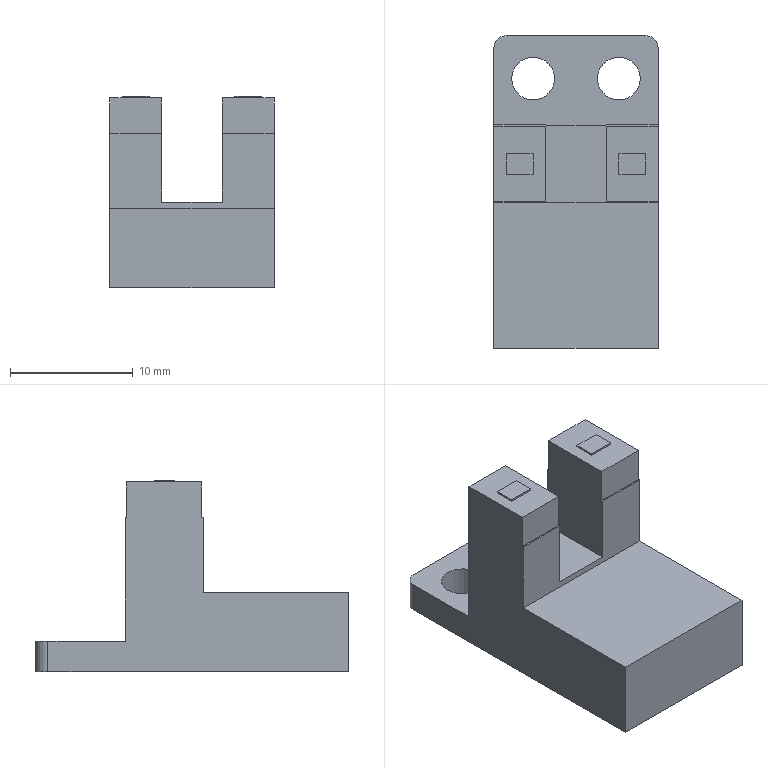Part | SolidWorks | features BaseBody 1 | 1 solid | 38 faces | box 13.4 x 25.5 x 15.65 mm | volume 2274 mm3 | plane 32 | cylinder 6 | commonest cylinder face diameters 3.5 x4 2 x2
STEP:
#1=CARTESIAN_POINT('',(304.797,1020.806,-399.345));
#2=VERTEX_POINT('',#1);
#3=CARTESIAN_POINT('',(301.297,1020.806,-399.345));
#4=VERTEX_POINT('',#3);
#5=CARTESIAN_POINT('',(303.047,1020.806,-399.345));
#6=DIRECTION('',(0.,0.,-1.));
#7=DIRECTION('',(-1.,0.,0.));
#8=AXIS2_PLACEMENT_3D('',#5,#6,#7);
#9=CIRCLE('',#8,1.75);
#10=EDGE_CURVE('',#2,#4,#9,.T.);
#11=ORIENTED_EDGE('',*,*,#10,.F.);
#12=CARTESIAN_POINT('',(304.797,1020.806,-401.845));
#13=VERTEX_POINT('',#12);
#14=CARTESIAN_POINT('',(304.797,1020.806,-344.345));
#15=DIRECTION('',(0.,0.,-1.));
#16=VECTOR('',#15,1000.);
#17=LINE('',#14,#16);
#18=EDGE_CURVE('',#2,#13,#17,.T.);
#19=ORIENTED_EDGE('',*,*,#18,.T.);
#20=CARTESIAN_POINT('',(301.297,1020.806,-401.845));
#21=VERTEX_POINT('',#20);
#22=CARTESIAN_POINT('',(303.047,1020.806,-401.845));
#23=DIRECTION('',(0.,0.,1.));
#24=DIRECTION('',(-1.,0.,0.));
#25=AXIS2_PLACEMENT_3D('',#22,#23,#24);
#26=CIRCLE('',#25,1.75);
#27=EDGE_CURVE('',#21,#13,#26,.T.);
#28=ORIENTED_EDGE('',*,*,#27,.F.);
#29=CARTESIAN_POINT('',(301.297,1020.806,-344.345));
#30=DIRECTION('',(0.,0.,-1.));
#31=VECTOR('',#30,1000.);
#32=LINE('',#29,#31);
#33=EDGE_CURVE('',#4,#21,#32,.T.);
#34=ORIENTED_EDGE('',*,*,#33,.F.);
#35=EDGE_LOOP('',(#11,#19,#28,#34));
#36=FACE_OUTER_BOUND('',#35,.T.);
#37=CARTESIAN_POINT('',(303.047,1020.806,-344.345));
#38=DIRECTION('',(0.,0.,-1.));
#39=DIRECTION('',(-1.,0.,0.));
#40=AXIS2_PLACEMENT_3D('',#37,#38,#39);
#41=CYLINDRICAL_SURFACE('',#40,1.75);
#42=ADVANCED_FACE('',(#36),#41,.F.);
#43=CARTESIAN_POINT('',(297.797,1020.806,-399.345));
#44=VERTEX_POINT('',#43);
#45=CARTESIAN_POINT('',(294.297,1020.806,-399.345));
#46=VERTEX_POINT('',#45);
#47=CARTESIAN_POINT('',(296.047,1020.806,-399.345));
#48=DIRECTION('',(0.,0.,-1.));
#49=DIRECTION('',(-1.,0.,0.));
#50=AXIS2_PLACEMENT_3D('',#47,#48,#49);
#51=CIRCLE('',#50,1.75);
#52=EDGE_CURVE('',#44,#46,#51,.T.);
#53=ORIENTED_EDGE('',*,*,#52,.F.);
#54=CARTESIAN_POINT('',(297.797,1020.806,-401.845));
#55=VERTEX_POINT('',#54);
#56=CARTESIAN_POINT('',(297.797,1020.806,-344.345));
#57=DIRECTION('',(0.,0.,-1.));
#58=VECTOR('',#57,1000.);
#59=LINE('',#56,#58);
#60=EDGE_CURVE('',#44,#55,#59,.T.);
#61=ORIENTED_EDGE('',*,*,#60,.T.);
#62=CARTESIAN_POINT('',(294.297,1020.806,-401.845));
#63=VERTEX_POINT('',#62);
#64=CARTESIAN_POINT('',(296.047,1020.806,-401.845));
#65=DIRECTION('',(0.,0.,1.));
#66=DIRECTION('',(-1.,0.,0.));
#67=AXIS2_PLACEMENT_3D('',#64,#65,#66);
#68=CIRCLE('',#67,1.75);
#69=EDGE_CURVE('',#63,#55,#68,.T.);
#70=ORIENTED_EDGE('',*,*,#69,.F.);
#71=CARTESIAN_POINT('',(294.297,1020.806,-344.345));
#72=DIRECTION('',(0.,0.,-1.));
#73=VECTOR('',#72,1000.);
#74=LINE('',#71,#73);
#75=EDGE_CURVE('',#46,#63,#74,.T.);
#76=ORIENTED_EDGE('',*,*,#75,.F.);
#77=EDGE_LOOP('',(#53,#61,#70,#76));
#78=FACE_OUTER_BOUND('',#77,.T.);
#79=CARTESIAN_POINT('',(296.047,1020.806,-344.345));
#80=DIRECTION('',(0.,0.,-1.));
#81=DIRECTION('',(-1.,0.,0.));
#82=AXIS2_PLACEMENT_3D('',#79,#80,#81);
#83=CYLINDRICAL_SURFACE('',#82,1.75);
#84=ADVANCED_FACE('',(#78),#83,.F.);
#85=ORIENTED_EDGE('',*,*,#27,.T.);
#86=CARTESIAN_POINT('',(303.047,1020.806,-401.845));
#87=DIRECTION('',(0.,0.,1.));
#88=DIRECTION('',(-1.,0.,0.));
#89=AXIS2_PLACEMENT_3D('',#86,#87,#88);
#90=CIRCLE('',#89,1.75);
#91=EDGE_CURVE('',#13,#21,#90,.T.);
#92=ORIENTED_EDGE('',*,*,#91,.T.);
#93=EDGE_LOOP('',(#85,#92));
#94=FACE_BOUND('',#93,.T.);
#95=ORIENTED_EDGE('',*,*,#69,.T.);
#96=CARTESIAN_POINT('',(296.047,1020.806,-401.845));
#97=DIRECTION('',(0.,0.,1.));
#98=DIRECTION('',(-1.,0.,0.));
#99=AXIS2_PLACEMENT_3D('',#96,#97,#98);
#100=CIRCLE('',#99,1.75);
#101=EDGE_CURVE('',#55,#63,#100,.T.);
#102=ORIENTED_EDGE('',*,*,#101,.T.);
#103=EDGE_LOOP('',(#95,#102));
#104=FACE_BOUND('',#103,.T.);
#105=CARTESIAN_POINT('',(292.847,1023.306,-401.845));
#106=VERTEX_POINT('',#105);
#107=CARTESIAN_POINT('',(293.847,1024.306,-401.845));
#108=VERTEX_POINT('',#107);
#109=CARTESIAN_POINT('',(293.847,1023.306,-401.845));
#110=DIRECTION('',(0.,0.,-1.));
#111=DIRECTION('',(1.,0.,0.));
#112=AXIS2_PLACEMENT_3D('',#109,#110,#111);
#113=CIRCLE('',#112,1.);
#114=EDGE_CURVE('',#106,#108,#113,.T.);
#115=ORIENTED_EDGE('',*,*,#114,.T.);
#116=CARTESIAN_POINT('',(305.247,1024.306,-401.845));
#117=VERTEX_POINT('',#116);
#118=CARTESIAN_POINT('',(306.247,1024.306,-401.845));
#119=DIRECTION('',(1.,0.,0.));
#120=VECTOR('',#119,1000.);
#121=LINE('',#118,#120);
#122=EDGE_CURVE('',#108,#117,#121,.T.);
#123=ORIENTED_EDGE('',*,*,#122,.T.);
#124=CARTESIAN_POINT('',(306.247,1023.306,-401.845));
#125=VERTEX_POINT('',#124);
#126=CARTESIAN_POINT('',(305.247,1023.306,-401.845));
#127=DIRECTION('',(0.,0.,-1.));
#128=DIRECTION('',(-1.,0.,0.));
#129=AXIS2_PLACEMENT_3D('',#126,#127,#128);
#130=CIRCLE('',#129,1.);
#131=EDGE_CURVE('',#117,#125,#130,.T.);
#132=ORIENTED_EDGE('',*,*,#131,.T.);
#133=CARTESIAN_POINT('',(306.247,998.806,-401.845));
#134=VERTEX_POINT('',#133);
#135=CARTESIAN_POINT('',(306.247,998.806,-401.845));
#136=DIRECTION('',(0.,-1.,0.));
#137=VECTOR('',#136,1000.);
#138=LINE('',#135,#137);
#139=EDGE_CURVE('',#125,#134,#138,.T.);
#140=ORIENTED_EDGE('',*,*,#139,.T.);
#141=CARTESIAN_POINT('',(292.847,998.806,-401.845));
#142=VERTEX_POINT('',#141);
#143=CARTESIAN_POINT('',(306.247,998.806,-401.845));
#144=DIRECTION('',(-1.,0.,0.));
#145=VECTOR('',#144,1000.);
#146=LINE('',#143,#145);
#147=EDGE_CURVE('',#134,#142,#146,.T.);
#148=ORIENTED_EDGE('',*,*,#147,.T.);
#149=CARTESIAN_POINT('',(292.847,998.806,-401.845));
#150=DIRECTION('',(0.,1.,0.));
#151=VECTOR('',#150,1000.);
#152=LINE('',#149,#151);
#153=EDGE_CURVE('',#142,#106,#152,.T.);
#154=ORIENTED_EDGE('',*,*,#153,.T.);
#155=EDGE_LOOP('',(#115,#123,#132,#140,#148,#154));
#156=FACE_OUTER_BOUND('',#155,.T.);
#157=CARTESIAN_POINT('',(306.247,998.806,-401.845));
#158=DIRECTION('',(0.,0.,-1.));
#159=DIRECTION('',(-1.,0.,0.));
#160=AXIS2_PLACEMENT_3D('',#157,#158,#159);
#161=PLANE('',#160);
#162=ADVANCED_FACE('',(#94,#104,#156),#161,.T.);
#163=ORIENTED_EDGE('',*,*,#18,.F.);
#164=CARTESIAN_POINT('',(303.047,1020.806,-399.345));
#165=DIRECTION('',(0.,0.,-1.));
#166=DIRECTION('',(-1.,0.,0.));
#167=AXIS2_PLACEMENT_3D('',#164,#165,#166);
#168=CIRCLE('',#167,1.75);
#169=EDGE_CURVE('',#4,#2,#168,.T.);
#170=ORIENTED_EDGE('',*,*,#169,.F.);
#171=ORIENTED_EDGE('',*,*,#33,.T.);
#172=ORIENTED_EDGE('',*,*,#91,.F.);
#173=EDGE_LOOP('',(#163,#170,#171,#172));
#174=FACE_OUTER_BOUND('',#173,.T.);
#175=CARTESIAN_POINT('',(303.047,1020.806,-344.345));
#176=DIRECTION('',(0.,0.,-1.));
#177=DIRECTION('',(-1.,0.,0.));
#178=AXIS2_PLACEMENT_3D('',#175,#176,#177);
#179=CYLINDRICAL_SURFACE('',#178,1.75);
#180=ADVANCED_FACE('',(#174),#179,.F.);
#181=ORIENTED_EDGE('',*,*,#60,.F.);
#182=CARTESIAN_POINT('',(296.047,1020.806,-399.345));
#183=DIRECTION('',(0.,0.,-1.));
#184=DIRECTION('',(-1.,0.,0.));
#185=AXIS2_PLACEMENT_3D('',#182,#183,#184);
#186=CIRCLE('',#185,1.75);
#187=EDGE_CURVE('',#46,#44,#186,.T.);
#188=ORIENTED_EDGE('',*,*,#187,.F.);
#189=ORIENTED_EDGE('',*,*,#75,.T.);
#190=ORIENTED_EDGE('',*,*,#101,.F.);
#191=EDGE_LOOP('',(#181,#188,#189,#190));
#192=FACE_OUTER_BOUND('',#191,.T.);
#193=CARTESIAN_POINT('',(296.047,1020.806,-344.345));
#194=DIRECTION('',(0.,0.,-1.));
#195=DIRECTION('',(-1.,0.,0.));
#196=AXIS2_PLACEMENT_3D('',#193,#194,#195);
#197=CYLINDRICAL_SURFACE('',#196,1.75);
#198=ADVANCED_FACE('',(#192),#197,.F.);
#199=CARTESIAN_POINT('',(293.847,1024.306,-399.345));
#200=VERTEX_POINT('',#199);
#201=CARTESIAN_POINT('',(293.847,1024.306,-444.345));
#202=DIRECTION('',(0.,0.,1.));
#203=VECTOR('',#202,1000.);
#204=LINE('',#201,#203);
#205=EDGE_CURVE('',#108,#200,#204,.T.);
#206=ORIENTED_EDGE('',*,*,#205,.T.);
#207=CARTESIAN_POINT('',(305.247,1024.306,-399.345));
#208=VERTEX_POINT('',#207);
#209=CARTESIAN_POINT('',(357.247,1024.306,-399.345));
#210=DIRECTION('',(1.,0.,0.));
#211=VECTOR('',#210,1000.);
#212=LINE('',#209,#211);
#213=EDGE_CURVE('',#200,#208,#212,.T.);
#214=ORIENTED_EDGE('',*,*,#213,.T.);
#215=CARTESIAN_POINT('',(305.247,1024.306,-444.345));
#216=DIRECTION('',(0.,0.,-1.));
#217=VECTOR('',#216,1000.);
#218=LINE('',#215,#217);
#219=EDGE_CURVE('',#208,#117,#218,.T.);
#220=ORIENTED_EDGE('',*,*,#219,.T.);
#221=ORIENTED_EDGE('',*,*,#122,.F.);
#222=EDGE_LOOP('',(#206,#214,#220,#221));
#223=FACE_OUTER_BOUND('',#222,.T.);
#224=CARTESIAN_POINT('',(357.247,1024.306,-444.345));
#225=DIRECTION('',(0.,1.,0.));
#226=DIRECTION('',(0.,0.,1.));
#227=AXIS2_PLACEMENT_3D('',#224,#225,#226);
#228=PLANE('',#227);
#229=ADVANCED_FACE('',(#223),#228,.T.);
#230=ORIENTED_EDGE('',*,*,#205,.F.);
#231=ORIENTED_EDGE('',*,*,#114,.F.);
#232=CARTESIAN_POINT('',(292.847,1023.306,-399.345));
#233=VERTEX_POINT('',#232);
#234=CARTESIAN_POINT('',(292.847,1023.306,-444.345));
#235=DIRECTION('',(0.,0.,1.));
#236=VECTOR('',#235,1000.);
#237=LINE('',#234,#236);
#238=EDGE_CURVE('',#106,#233,#237,.T.);
#239=ORIENTED_EDGE('',*,*,#238,.T.);
#240=CARTESIAN_POINT('',(293.847,1023.306,-399.345));
#241=DIRECTION('',(0.,0.,-1.));
#242=DIRECTION('',(1.,0.,0.));
#243=AXIS2_PLACEMENT_3D('',#240,#241,#242);
#244=CIRCLE('',#243,1.);
#245=EDGE_CURVE('',#233,#200,#244,.T.);
#246=ORIENTED_EDGE('',*,*,#245,.T.);
#247=EDGE_LOOP('',(#230,#231,#239,#246));
#248=FACE_OUTER_BOUND('',#247,.T.);
#249=CARTESIAN_POINT('',(293.847,1023.306,-444.345));
#250=DIRECTION('',(0.,0.,1.));
#251=DIRECTION('',(1.,0.,0.));
#252=AXIS2_PLACEMENT_3D('',#249,#250,#251);
#253=CYLINDRICAL_SURFACE('',#252,1.);
#254=ADVANCED_FACE('',(#248),#253,.T.);
#255=CARTESIAN_POINT('',(292.847,1017.006,-389.245));
#256=VERTEX_POINT('',#255);
#257=CARTESIAN_POINT('',(292.847,1017.006,-399.345));
#258=VERTEX_POINT('',#257);
#259=CARTESIAN_POINT('',(292.847,1017.006,-401.845));
#260=DIRECTION('',(0.,0.,-1.));
#261=VECTOR('',#260,1000.);
#262=LINE('',#259,#261);
#263=EDGE_CURVE('',#256,#258,#262,.T.);
#264=ORIENTED_EDGE('',*,*,#263,.T.);
#265=CARTESIAN_POINT('',(292.847,998.806,-399.345));
#266=DIRECTION('',(0.,1.,0.));
#267=VECTOR('',#266,1000.);
#268=LINE('',#265,#267);
#269=EDGE_CURVE('',#258,#233,#268,.T.);
#270=ORIENTED_EDGE('',*,*,#269,.T.);
#271=ORIENTED_EDGE('',*,*,#238,.F.);
#272=ORIENTED_EDGE('',*,*,#153,.F.);
#273=CARTESIAN_POINT('',(292.847,998.806,-395.345));
#274=VERTEX_POINT('',#273);
#275=CARTESIAN_POINT('',(292.847,998.806,-401.845));
#276=DIRECTION('',(0.,0.,1.));
#277=VECTOR('',#276,1000.);
#278=LINE('',#275,#277);
#279=EDGE_CURVE('',#142,#274,#278,.T.);
#280=ORIENTED_EDGE('',*,*,#279,.T.);
#281=CARTESIAN_POINT('',(292.847,1010.656,-395.345));
#282=VERTEX_POINT('',#281);
#283=CARTESIAN_POINT('',(292.847,998.806,-395.345));
#284=DIRECTION('',(0.,1.,0.));
#285=VECTOR('',#284,1000.);
#286=LINE('',#283,#285);
#287=EDGE_CURVE('',#274,#282,#286,.T.);
#288=ORIENTED_EDGE('',*,*,#287,.T.);
#289=CARTESIAN_POINT('',(292.847,1010.656,-389.245));
#290=VERTEX_POINT('',#289);
#291=CARTESIAN_POINT('',(292.847,1010.656,-401.845));
#292=DIRECTION('',(0.,0.,1.));
#293=VECTOR('',#292,1000.);
#294=LINE('',#291,#293);
#295=EDGE_CURVE('',#282,#290,#294,.T.);
#296=ORIENTED_EDGE('',*,*,#295,.T.);
#297=CARTESIAN_POINT('',(292.847,1010.756,-389.245));
#298=VERTEX_POINT('',#297);
#299=CARTESIAN_POINT('',(292.847,998.806,-389.245));
#300=DIRECTION('',(0.,1.,0.));
#301=VECTOR('',#300,1000.);
#302=LINE('',#299,#301);
#303=EDGE_CURVE('',#290,#298,#302,.T.);
#304=ORIENTED_EDGE('',*,*,#303,.T.);
#305=CARTESIAN_POINT('',(292.847,1010.756,-386.345));
#306=VERTEX_POINT('',#305);
#307=CARTESIAN_POINT('',(292.847,1010.756,-401.845));
#308=DIRECTION('',(0.,0.,1.));
#309=VECTOR('',#308,1000.);
#310=LINE('',#307,#309);
#311=EDGE_CURVE('',#298,#306,#310,.T.);
#312=ORIENTED_EDGE('',*,*,#311,.T.);
#313=CARTESIAN_POINT('',(292.847,1016.906,-386.345));
#314=VERTEX_POINT('',#313);
#315=CARTESIAN_POINT('',(292.847,998.806,-386.345));
#316=DIRECTION('',(0.,1.,0.));
#317=VECTOR('',#316,1000.);
#318=LINE('',#315,#317);
#319=EDGE_CURVE('',#306,#314,#318,.T.);
#320=ORIENTED_EDGE('',*,*,#319,.T.);
#321=CARTESIAN_POINT('',(292.847,1016.906,-389.245));
#322=VERTEX_POINT('',#321);
#323=CARTESIAN_POINT('',(292.847,1016.906,-401.845));
#324=DIRECTION('',(0.,0.,-1.));
#325=VECTOR('',#324,1000.);
#326=LINE('',#323,#325);
#327=EDGE_CURVE('',#314,#322,#326,.T.);
#328=ORIENTED_EDGE('',*,*,#327,.T.);
#329=CARTESIAN_POINT('',(292.847,998.806,-389.245));
#330=DIRECTION('',(0.,1.,0.));
#331=VECTOR('',#330,1000.);
#332=LINE('',#329,#331);
#333=EDGE_CURVE('',#322,#256,#332,.T.);
#334=ORIENTED_EDGE('',*,*,#333,.T.);
#335=EDGE_LOOP('',(#264,#270,#271,#272,#280,#288,#296,#304,#312,#320,#328,#334));
#336=FACE_OUTER_BOUND('',#335,.T.);
#337=CARTESIAN_POINT('',(292.847,998.806,-401.845));
#338=DIRECTION('',(-1.,0.,0.));
#339=DIRECTION('',(0.,0.,1.));
#340=AXIS2_PLACEMENT_3D('',#337,#338,#339);
#341=PLANE('',#340);
#342=ADVANCED_FACE('',(#336),#341,.T.);
#343=ORIENTED_EDGE('',*,*,#279,.F.);
#344=ORIENTED_EDGE('',*,*,#147,.F.);
#345=CARTESIAN_POINT('',(306.247,998.806,-395.345));
#346=VERTEX_POINT('',#345);
#347=CARTESIAN_POINT('',(306.247,998.806,-444.345));
#348=DIRECTION('',(0.,0.,-1.));
#349=VECTOR('',#348,1000.);
#350=LINE('',#347,#349);
#351=EDGE_CURVE('',#346,#134,#350,.T.);
#352=ORIENTED_EDGE('',*,*,#351,.F.);
#353=CARTESIAN_POINT('',(357.247,998.806,-395.345));
#354=DIRECTION('',(1.,0.,0.));
#355=VECTOR('',#354,1000.);
#356=LINE('',#353,#355);
#357=EDGE_CURVE('',#274,#346,#356,.T.);
#358=ORIENTED_EDGE('',*,*,#357,.F.);
#359=EDGE_LOOP('',(#343,#344,#352,#358));
#360=FACE_OUTER_BOUND('',#359,.T.);
#361=CARTESIAN_POINT('',(357.247,998.806,-444.345));
#362=DIRECTION('',(0.,1.,0.));
#363=DIRECTION('',(0.,0.,1.));
#364=AXIS2_PLACEMENT_3D('',#361,#362,#363);
#365=PLANE('',#364);
#366=ADVANCED_FACE('',(#360),#365,.F.);
#367=ORIENTED_EDGE('',*,*,#351,.T.);
#368=ORIENTED_EDGE('',*,*,#139,.F.);
#369=CARTESIAN_POINT('',(306.247,1023.306,-399.345));
#370=VERTEX_POINT('',#369);
#371=CARTESIAN_POINT('',(306.247,1023.306,-386.345));
#372=DIRECTION('',(0.,0.,1.));
#373=VECTOR('',#372,1000.);
#374=LINE('',#371,#373);
#375=EDGE_CURVE('',#125,#370,#374,.T.);
#376=ORIENTED_EDGE('',*,*,#375,.T.);
#377=CARTESIAN_POINT('',(306.247,1017.006,-399.345));
#378=VERTEX_POINT('',#377);
#379=CARTESIAN_POINT('',(306.247,998.806,-399.345));
#380=DIRECTION('',(0.,-1.,0.));
#381=VECTOR('',#380,1000.);
#382=LINE('',#379,#381);
#383=EDGE_CURVE('',#370,#378,#382,.T.);
#384=ORIENTED_EDGE('',*,*,#383,.T.);
#385=CARTESIAN_POINT('',(306.247,1017.006,-389.245));
#386=VERTEX_POINT('',#385);
#387=CARTESIAN_POINT('',(306.247,1017.006,-386.345));
#388=DIRECTION('',(0.,0.,1.));
#389=VECTOR('',#388,1000.);
#390=LINE('',#387,#389);
#391=EDGE_CURVE('',#378,#386,#390,.T.);
#392=ORIENTED_EDGE('',*,*,#391,.T.);
#393=CARTESIAN_POINT('',(306.247,1016.906,-389.245));
#394=VERTEX_POINT('',#393);
#395=CARTESIAN_POINT('',(306.247,998.806,-389.245));
#396=DIRECTION('',(0.,-1.,0.));
#397=VECTOR('',#396,1000.);
#398=LINE('',#395,#397);
#399=EDGE_CURVE('',#386,#394,#398,.T.);
#400=ORIENTED_EDGE('',*,*,#399,.T.);
#401=CARTESIAN_POINT('',(306.247,1016.906,-386.345));
#402=VERTEX_POINT('',#401);
#403=CARTESIAN_POINT('',(306.247,1016.906,-386.345));
#404=DIRECTION('',(0.,0.,1.));
#405=VECTOR('',#404,1000.);
#406=LINE('',#403,#405);
#407=EDGE_CURVE('',#394,#402,#406,.T.);
#408=ORIENTED_EDGE('',*,*,#407,.T.);
#409=CARTESIAN_POINT('',(306.247,1010.756,-386.345));
#410=VERTEX_POINT('',#409);
#411=CARTESIAN_POINT('',(306.247,998.806,-386.345));
#412=DIRECTION('',(0.,-1.,0.));
#413=VECTOR('',#412,1000.);
#414=LINE('',#411,#413);
#415=EDGE_CURVE('',#402,#410,#414,.T.);
#416=ORIENTED_EDGE('',*,*,#415,.T.);
#417=CARTESIAN_POINT('',(306.247,1010.756,-389.245));
#418=VERTEX_POINT('',#417);
#419=CARTESIAN_POINT('',(306.247,1010.756,-386.345));
#420=DIRECTION('',(0.,0.,-1.));
#421=VECTOR('',#420,1000.);
#422=LINE('',#419,#421);
#423=EDGE_CURVE('',#410,#418,#422,.T.);
#424=ORIENTED_EDGE('',*,*,#423,.T.);
#425=CARTESIAN_POINT('',(306.247,1010.656,-389.245));
#426=VERTEX_POINT('',#425);
#427=CARTESIAN_POINT('',(306.247,998.806,-389.245));
#428=DIRECTION('',(0.,-1.,0.));
#429=VECTOR('',#428,1000.);
#430=LINE('',#427,#429);
#431=EDGE_CURVE('',#418,#426,#430,.T.);
#432=ORIENTED_EDGE('',*,*,#431,.T.);
#433=CARTESIAN_POINT('',(306.247,1010.656,-395.345));
#434=VERTEX_POINT('',#433);
#435=CARTESIAN_POINT('',(306.247,1010.656,-386.345));
#436=DIRECTION('',(0.,0.,-1.));
#437=VECTOR('',#436,1000.);
#438=LINE('',#435,#437);
#439=EDGE_CURVE('',#426,#434,#438,.T.);
#440=ORIENTED_EDGE('',*,*,#439,.T.);
#441=CARTESIAN_POINT('',(306.247,998.806,-395.345));
#442=DIRECTION('',(0.,-1.,0.));
#443=VECTOR('',#442,1000.);
#444=LINE('',#441,#443);
#445=EDGE_CURVE('',#434,#346,#444,.T.);
#446=ORIENTED_EDGE('',*,*,#445,.T.);
#447=EDGE_LOOP('',(#367,#368,#376,#384,#392,#400,#408,#416,#424,#432,#440,#446));
#448=FACE_OUTER_BOUND('',#447,.T.);
#449=CARTESIAN_POINT('',(306.247,998.806,-386.345));
#450=DIRECTION('',(1.,0.,0.));
#451=DIRECTION('',(0.,0.,-1.));
#452=AXIS2_PLACEMENT_3D('',#449,#450,#451);
#453=PLANE('',#452);
#454=ADVANCED_FACE('',(#448),#453,.T.);
#455=ORIENTED_EDGE('',*,*,#219,.F.);
#456=CARTESIAN_POINT('',(305.247,1023.306,-399.345));
#457=DIRECTION('',(0.,0.,-1.));
#458=DIRECTION('',(-1.,0.,0.));
#459=AXIS2_PLACEMENT_3D('',#456,#457,#458);
#460=CIRCLE('',#459,1.);
#461=EDGE_CURVE('',#208,#370,#460,.T.);
#462=ORIENTED_EDGE('',*,*,#461,.T.);
#463=ORIENTED_EDGE('',*,*,#375,.F.);
#464=ORIENTED_EDGE('',*,*,#131,.F.);
#465=EDGE_LOOP('',(#455,#462,#463,#464));
#466=FACE_OUTER_BOUND('',#465,.T.);
#467=CARTESIAN_POINT('',(305.247,1023.306,-444.345));
#468=DIRECTION('',(0.,0.,-1.));
#469=DIRECTION('',(-1.,0.,0.));
#470=AXIS2_PLACEMENT_3D('',#467,#468,#469);
#471=CYLINDRICAL_SURFACE('',#470,1.);
#472=ADVANCED_FACE('',(#466),#471,.T.);
#473=ORIENTED_EDGE('',*,*,#169,.T.);
#474=ORIENTED_EDGE('',*,*,#10,.T.);
#475=EDGE_LOOP('',(#473,#474));
#476=FACE_BOUND('',#475,.T.);
#477=ORIENTED_EDGE('',*,*,#187,.T.);
#478=ORIENTED_EDGE('',*,*,#52,.T.);
#479=EDGE_LOOP('',(#477,#478));
#480=FACE_BOUND('',#479,.T.);
#481=ORIENTED_EDGE('',*,*,#213,.F.);
#482=ORIENTED_EDGE('',*,*,#245,.F.);
#483=ORIENTED_EDGE('',*,*,#269,.F.);
#484=CARTESIAN_POINT('',(257.247,1017.006,-399.345));
#485=DIRECTION('',(-1.,0.,0.));
#486=VECTOR('',#485,1000.);
#487=LINE('',#484,#486);
#488=EDGE_CURVE('',#378,#258,#487,.T.);
#489=ORIENTED_EDGE('',*,*,#488,.F.);
#490=ORIENTED_EDGE('',*,*,#383,.F.);
#491=ORIENTED_EDGE('',*,*,#461,.F.);
#492=EDGE_LOOP('',(#481,#482,#483,#489,#490,#491));
#493=FACE_OUTER_BOUND('',#492,.T.);
#494=CARTESIAN_POINT('',(257.247,1017.006,-399.345));
#495=DIRECTION('',(0.,0.,-1.));
#496=DIRECTION('',(-1.,0.,0.));
#497=AXIS2_PLACEMENT_3D('',#494,#495,#496);
#498=PLANE('',#497);
#499=ADVANCED_FACE('',(#476,#480,#493),#498,.F.);
#500=ORIENTED_EDGE('',*,*,#263,.F.);
#501=CARTESIAN_POINT('',(297.063,1017.006,-389.245));
#502=VERTEX_POINT('',#501);
#503=CARTESIAN_POINT('',(257.247,1017.006,-389.245));
#504=DIRECTION('',(-1.,0.,0.));
#505=VECTOR('',#504,1000.);
#506=LINE('',#503,#505);
#507=EDGE_CURVE('',#502,#256,#506,.T.);
#508=ORIENTED_EDGE('',*,*,#507,.F.);
#509=CARTESIAN_POINT('',(297.063,1017.006,-394.845));
#510=VERTEX_POINT('',#509);
#511=CARTESIAN_POINT('',(297.063,1017.006,-389.245));
#512=DIRECTION('',(0.,0.,1.));
#513=VECTOR('',#512,1000.);
#514=LINE('',#511,#513);
#515=EDGE_CURVE('',#510,#502,#514,.T.);
#516=ORIENTED_EDGE('',*,*,#515,.F.);
#517=CARTESIAN_POINT('',(302.031,1017.006,-394.845));
#518=VERTEX_POINT('',#517);
#519=CARTESIAN_POINT('',(257.247,1017.006,-394.845));
#520=DIRECTION('',(-1.,0.,0.));
#521=VECTOR('',#520,1000.);
#522=LINE('',#519,#521);
#523=EDGE_CURVE('',#518,#510,#522,.T.);
#524=ORIENTED_EDGE('',*,*,#523,.F.);
#525=CARTESIAN_POINT('',(302.031,1017.006,-389.245));
#526=VERTEX_POINT('',#525);
#527=CARTESIAN_POINT('',(302.031,1017.006,-389.245));
#528=DIRECTION('',(0.,0.,-1.));
#529=VECTOR('',#528,1000.);
#530=LINE('',#527,#529);
#531=EDGE_CURVE('',#526,#518,#530,.T.);
#532=ORIENTED_EDGE('',*,*,#531,.F.);
#533=CARTESIAN_POINT('',(257.247,1017.006,-389.245));
#534=DIRECTION('',(-1.,0.,0.));
#535=VECTOR('',#534,1000.);
#536=LINE('',#533,#535);
#537=EDGE_CURVE('',#386,#526,#536,.T.);
#538=ORIENTED_EDGE('',*,*,#537,.F.);
#539=ORIENTED_EDGE('',*,*,#391,.F.);
#540=ORIENTED_EDGE('',*,*,#488,.T.);
#541=EDGE_LOOP('',(#500,#508,#516,#524,#532,#538,#539,#540));
#542=FACE_OUTER_BOUND('',#541,.T.);
#543=CARTESIAN_POINT('',(257.247,1017.006,-389.245));
#544=DIRECTION('',(0.,-1.,0.));
#545=DIRECTION('',(0.,0.,-1.));
#546=AXIS2_PLACEMENT_3D('',#543,#544,#545);
#547=PLANE('',#546);
#548=ADVANCED_FACE('',(#542),#547,.F.);
#549=CARTESIAN_POINT('',(297.063,1016.906,-389.245));
#550=VERTEX_POINT('',#549);
#551=CARTESIAN_POINT('',(297.063,1016.906,-389.245));
#552=DIRECTION('',(0.,-1.,0.));
#553=VECTOR('',#552,1000.);
#554=LINE('',#551,#553);
#555=EDGE_CURVE('',#502,#550,#554,.T.);
#556=ORIENTED_EDGE('',*,*,#555,.F.);
#557=ORIENTED_EDGE('',*,*,#507,.T.);
#558=ORIENTED_EDGE('',*,*,#333,.F.);
#559=CARTESIAN_POINT('',(257.247,1016.906,-389.245));
#560=DIRECTION('',(-1.,0.,0.));
#561=VECTOR('',#560,1000.);
#562=LINE('',#559,#561);
#563=EDGE_CURVE('',#550,#322,#562,.T.);
#564=ORIENTED_EDGE('',*,*,#563,.F.);
#565=EDGE_LOOP('',(#556,#557,#558,#564));
#566=FACE_OUTER_BOUND('',#565,.T.);
#567=CARTESIAN_POINT('',(257.247,1016.906,-389.245));
#568=DIRECTION('',(0.,0.,-1.));
#569=DIRECTION('',(-1.,0.,0.));
#570=AXIS2_PLACEMENT_3D('',#567,#568,#569);
#571=PLANE('',#570);
#572=ADVANCED_FACE('',(#566),#571,.F.);
#573=CARTESIAN_POINT('',(297.063,1016.906,-386.345));
#574=VERTEX_POINT('',#573);
#575=CARTESIAN_POINT('',(297.063,1016.906,-386.345));
#576=DIRECTION('',(0.,0.,1.));
#577=VECTOR('',#576,1000.);
#578=LINE('',#575,#577);
#579=EDGE_CURVE('',#550,#574,#578,.T.);
#580=ORIENTED_EDGE('',*,*,#579,.F.);
#581=ORIENTED_EDGE('',*,*,#563,.T.);
#582=ORIENTED_EDGE('',*,*,#327,.F.);
#583=CARTESIAN_POINT('',(257.247,1016.906,-386.345));
#584=DIRECTION('',(-1.,0.,0.));
#585=VECTOR('',#584,1000.);
#586=LINE('',#583,#585);
#587=EDGE_CURVE('',#574,#314,#586,.T.);
#588=ORIENTED_EDGE('',*,*,#587,.F.);
#589=EDGE_LOOP('',(#580,#581,#582,#588));
#590=FACE_OUTER_BOUND('',#589,.T.);
#591=CARTESIAN_POINT('',(257.247,1016.906,-386.345));
#592=DIRECTION('',(0.,-1.,0.));
#593=DIRECTION('',(0.,0.,-1.));
#594=AXIS2_PLACEMENT_3D('',#591,#592,#593);
#595=PLANE('',#594);
#596=ADVANCED_FACE('',(#590),#595,.F.);
#597=CARTESIAN_POINT('',(293.847,1014.646,-386.345));
#598=VERTEX_POINT('',#597);
#599=CARTESIAN_POINT('',(296.047,1014.646,-386.345));
#600=VERTEX_POINT('',#599);
#601=CARTESIAN_POINT('',(296.047,1014.646,-386.345));
#602=DIRECTION('',(1.,0.,0.));
#603=VECTOR('',#602,1000.);
#604=LINE('',#601,#603);
#605=EDGE_CURVE('',#598,#600,#604,.T.);
#606=ORIENTED_EDGE('',*,*,#605,.T.);
#607=CARTESIAN_POINT('',(296.047,1012.966,-386.345));
#608=VERTEX_POINT('',#607);
#609=CARTESIAN_POINT('',(296.047,998.806,-386.345));
#610=DIRECTION('',(0.,-1.,0.));
#611=VECTOR('',#610,1000.);
#612=LINE('',#609,#611);
#613=EDGE_CURVE('',#600,#608,#612,.T.);
#614=ORIENTED_EDGE('',*,*,#613,.T.);
#615=CARTESIAN_POINT('',(293.847,1012.966,-386.345));
#616=VERTEX_POINT('',#615);
#617=CARTESIAN_POINT('',(296.047,1012.966,-386.345));
#618=DIRECTION('',(-1.,0.,0.));
#619=VECTOR('',#618,1000.);
#620=LINE('',#617,#619);
#621=EDGE_CURVE('',#608,#616,#620,.T.);
#622=ORIENTED_EDGE('',*,*,#621,.T.);
#623=CARTESIAN_POINT('',(293.847,998.806,-386.345));
#624=DIRECTION('',(0.,1.,0.));
#625=VECTOR('',#624,1000.);
#626=LINE('',#623,#625);
#627=EDGE_CURVE('',#616,#598,#626,.T.);
#628=ORIENTED_EDGE('',*,*,#627,.T.);
#629=EDGE_LOOP('',(#606,#614,#622,#628));
#630=FACE_BOUND('',#629,.T.);
#631=CARTESIAN_POINT('',(297.063,1010.756,-386.345));
#632=VERTEX_POINT('',#631);
#633=CARTESIAN_POINT('',(297.063,998.806,-386.345));
#634=DIRECTION('',(0.,1.,0.));
#635=VECTOR('',#634,1000.);
#636=LINE('',#633,#635);
#637=EDGE_CURVE('',#632,#574,#636,.T.);
#638=ORIENTED_EDGE('',*,*,#637,.T.);
#639=ORIENTED_EDGE('',*,*,#587,.T.);
#640=ORIENTED_EDGE('',*,*,#319,.F.);
#641=CARTESIAN_POINT('',(296.047,1010.756,-386.345));
#642=DIRECTION('',(1.,0.,0.));
#643=VECTOR('',#642,1000.);
#644=LINE('',#641,#643);
#645=EDGE_CURVE('',#306,#632,#644,.T.);
#646=ORIENTED_EDGE('',*,*,#645,.T.);
#647=EDGE_LOOP('',(#638,#639,#640,#646));
#648=FACE_OUTER_BOUND('',#647,.T.);
#649=CARTESIAN_POINT('',(296.047,998.806,-386.345));
#650=DIRECTION('',(0.,0.,1.));
#651=DIRECTION('',(1.,0.,0.));
#652=AXIS2_PLACEMENT_3D('',#649,#650,#651);
#653=PLANE('',#652);
#654=ADVANCED_FACE('',(#630,#648),#653,.T.);
#655=CARTESIAN_POINT('',(297.063,1010.756,-389.245));
#656=VERTEX_POINT('',#655);
#657=CARTESIAN_POINT('',(297.063,1010.756,-389.245));
#658=DIRECTION('',(0.,0.,-1.));
#659=VECTOR('',#658,1000.);
#660=LINE('',#657,#659);
#661=EDGE_CURVE('',#632,#656,#660,.T.);
#662=ORIENTED_EDGE('',*,*,#661,.F.);
#663=ORIENTED_EDGE('',*,*,#645,.F.);
#664=ORIENTED_EDGE('',*,*,#311,.F.);
#665=CARTESIAN_POINT('',(257.247,1010.756,-389.245));
#666=DIRECTION('',(-1.,0.,0.));
#667=VECTOR('',#666,1000.);
#668=LINE('',#665,#667);
#669=EDGE_CURVE('',#656,#298,#668,.T.);
#670=ORIENTED_EDGE('',*,*,#669,.F.);
#671=EDGE_LOOP('',(#662,#663,#664,#670));
#672=FACE_OUTER_BOUND('',#671,.T.);
#673=CARTESIAN_POINT('',(257.247,1010.756,-389.245));
#674=DIRECTION('',(0.,1.,0.));
#675=DIRECTION('',(0.,0.,1.));
#676=AXIS2_PLACEMENT_3D('',#673,#674,#675);
#677=PLANE('',#676);
#678=ADVANCED_FACE('',(#672),#677,.F.);
#679=CARTESIAN_POINT('',(297.063,1010.656,-389.245));
#680=VERTEX_POINT('',#679);
#681=CARTESIAN_POINT('',(297.063,1010.656,-389.245));
#682=DIRECTION('',(0.,-1.,0.));
#683=VECTOR('',#682,1000.);
#684=LINE('',#681,#683);
#685=EDGE_CURVE('',#656,#680,#684,.T.);
#686=ORIENTED_EDGE('',*,*,#685,.F.);
#687=ORIENTED_EDGE('',*,*,#669,.T.);
#688=ORIENTED_EDGE('',*,*,#303,.F.);
#689=CARTESIAN_POINT('',(257.247,1010.656,-389.245));
#690=DIRECTION('',(-1.,0.,0.));
#691=VECTOR('',#690,1000.);
#692=LINE('',#689,#691);
#693=EDGE_CURVE('',#680,#290,#692,.T.);
#694=ORIENTED_EDGE('',*,*,#693,.F.);
#695=EDGE_LOOP('',(#686,#687,#688,#694));
#696=FACE_OUTER_BOUND('',#695,.T.);
#697=CARTESIAN_POINT('',(257.247,1010.656,-389.245));
#698=DIRECTION('',(0.,0.,-1.));
#699=DIRECTION('',(-1.,0.,0.));
#700=AXIS2_PLACEMENT_3D('',#697,#698,#699);
#701=PLANE('',#700);
#702=ADVANCED_FACE('',(#696),#701,.F.);
#703=CARTESIAN_POINT('',(302.031,1010.656,-394.845));
#704=VERTEX_POINT('',#703);
#705=CARTESIAN_POINT('',(302.031,1010.656,-389.245));
#706=VERTEX_POINT('',#705);
#707=CARTESIAN_POINT('',(302.031,1010.656,-395.345));
#708=DIRECTION('',(0.,0.,1.));
#709=VECTOR('',#708,1000.);
#710=LINE('',#707,#709);
#711=EDGE_CURVE('',#704,#706,#710,.T.);
#712=ORIENTED_EDGE('',*,*,#711,.F.);
#713=CARTESIAN_POINT('',(297.063,1010.656,-394.845));
#714=VERTEX_POINT('',#713);
#715=CARTESIAN_POINT('',(257.247,1010.656,-394.845));
#716=DIRECTION('',(1.,0.,0.));
#717=VECTOR('',#716,1000.);
#718=LINE('',#715,#717);
#719=EDGE_CURVE('',#714,#704,#718,.T.);
#720=ORIENTED_EDGE('',*,*,#719,.F.);
#721=CARTESIAN_POINT('',(297.063,1010.656,-395.345));
#722=DIRECTION('',(0.,0.,-1.));
#723=VECTOR('',#722,1000.);
#724=LINE('',#721,#723);
#725=EDGE_CURVE('',#680,#714,#724,.T.);
#726=ORIENTED_EDGE('',*,*,#725,.F.);
#727=ORIENTED_EDGE('',*,*,#693,.T.);
#728=ORIENTED_EDGE('',*,*,#295,.F.);
#729=CARTESIAN_POINT('',(257.247,1010.656,-395.345));
#730=DIRECTION('',(-1.,0.,0.));
#731=VECTOR('',#730,1000.);
#732=LINE('',#729,#731);
#733=EDGE_CURVE('',#434,#282,#732,.T.);
#734=ORIENTED_EDGE('',*,*,#733,.F.);
#735=ORIENTED_EDGE('',*,*,#439,.F.);
#736=CARTESIAN_POINT('',(257.247,1010.656,-389.245));
#737=DIRECTION('',(1.,0.,0.));
#738=VECTOR('',#737,1000.);
#739=LINE('',#736,#738);
#740=EDGE_CURVE('',#706,#426,#739,.T.);
#741=ORIENTED_EDGE('',*,*,#740,.F.);
#742=EDGE_LOOP('',(#712,#720,#726,#727,#728,#734,#735,#741));
#743=FACE_OUTER_BOUND('',#742,.T.);
#744=CARTESIAN_POINT('',(257.247,1010.656,-395.345));
#745=DIRECTION('',(0.,1.,0.));
#746=DIRECTION('',(0.,0.,1.));
#747=AXIS2_PLACEMENT_3D('',#744,#745,#746);
#748=PLANE('',#747);
#749=ADVANCED_FACE('',(#743),#748,.F.);
#750=ORIENTED_EDGE('',*,*,#287,.F.);
#751=ORIENTED_EDGE('',*,*,#357,.T.);
#752=ORIENTED_EDGE('',*,*,#445,.F.);
#753=ORIENTED_EDGE('',*,*,#733,.T.);
#754=EDGE_LOOP('',(#750,#751,#752,#753));
#755=FACE_OUTER_BOUND('',#754,.T.);
#756=CARTESIAN_POINT('',(257.247,998.806,-395.345));
#757=DIRECTION('',(0.,0.,-1.));
#758=DIRECTION('',(-1.,0.,0.));
#759=AXIS2_PLACEMENT_3D('',#756,#757,#758);
#760=PLANE('',#759);
#761=ADVANCED_FACE('',(#755),#760,.F.);
#762=CARTESIAN_POINT('',(302.031,1010.756,-389.245));
#763=VERTEX_POINT('',#762);
#764=CARTESIAN_POINT('',(302.031,1010.656,-389.245));
#765=DIRECTION('',(0.,1.,0.));
#766=VECTOR('',#765,1000.);
#767=LINE('',#764,#766);
#768=EDGE_CURVE('',#706,#763,#767,.T.);
#769=ORIENTED_EDGE('',*,*,#768,.F.);
#770=ORIENTED_EDGE('',*,*,#740,.T.);
#771=ORIENTED_EDGE('',*,*,#431,.F.);
#772=CARTESIAN_POINT('',(257.247,1010.756,-389.245));
#773=DIRECTION('',(1.,0.,0.));
#774=VECTOR('',#773,1000.);
#775=LINE('',#772,#774);
#776=EDGE_CURVE('',#763,#418,#775,.T.);
#777=ORIENTED_EDGE('',*,*,#776,.F.);
#778=EDGE_LOOP('',(#769,#770,#771,#777));
#779=FACE_OUTER_BOUND('',#778,.T.);
#780=CARTESIAN_POINT('',(257.247,1010.656,-389.245));
#781=DIRECTION('',(0.,0.,-1.));
#782=DIRECTION('',(-1.,0.,0.));
#783=AXIS2_PLACEMENT_3D('',#780,#781,#782);
#784=PLANE('',#783);
#785=ADVANCED_FACE('',(#779),#784,.F.);
#786=CARTESIAN_POINT('',(302.031,1010.756,-386.345));
#787=VERTEX_POINT('',#786);
#788=CARTESIAN_POINT('',(302.031,1010.756,-389.245));
#789=DIRECTION('',(0.,0.,1.));
#790=VECTOR('',#789,1000.);
#791=LINE('',#788,#790);
#792=EDGE_CURVE('',#763,#787,#791,.T.);
#793=ORIENTED_EDGE('',*,*,#792,.F.);
#794=ORIENTED_EDGE('',*,*,#776,.T.);
#795=ORIENTED_EDGE('',*,*,#423,.F.);
#796=CARTESIAN_POINT('',(257.247,1010.756,-386.345));
#797=DIRECTION('',(1.,0.,0.));
#798=VECTOR('',#797,1000.);
#799=LINE('',#796,#798);
#800=EDGE_CURVE('',#787,#410,#799,.T.);
#801=ORIENTED_EDGE('',*,*,#800,.F.);
#802=EDGE_LOOP('',(#793,#794,#795,#801));
#803=FACE_OUTER_BOUND('',#802,.T.);
#804=CARTESIAN_POINT('',(257.247,1010.756,-389.245));
#805=DIRECTION('',(0.,1.,0.));
#806=DIRECTION('',(0.,0.,1.));
#807=AXIS2_PLACEMENT_3D('',#804,#805,#806);
#808=PLANE('',#807);
#809=ADVANCED_FACE('',(#803),#808,.F.);
#810=CARTESIAN_POINT('',(303.047,1014.646,-386.345));
#811=VERTEX_POINT('',#810);
#812=CARTESIAN_POINT('',(305.247,1014.646,-386.345));
#813=VERTEX_POINT('',#812);
#814=CARTESIAN_POINT('',(302.031,1014.646,-386.345));
#815=DIRECTION('',(1.,0.,0.));
#816=VECTOR('',#815,1000.);
#817=LINE('',#814,#816);
#818=EDGE_CURVE('',#811,#813,#817,.T.);
#819=ORIENTED_EDGE('',*,*,#818,.T.);
#820=CARTESIAN_POINT('',(305.247,1012.966,-386.345));
#821=VERTEX_POINT('',#820);
#822=CARTESIAN_POINT('',(305.247,998.806,-386.345));
#823=DIRECTION('',(0.,-1.,0.));
#824=VECTOR('',#823,1000.);
#825=LINE('',#822,#824);
#826=EDGE_CURVE('',#813,#821,#825,.T.);
#827=ORIENTED_EDGE('',*,*,#826,.T.);
#828=CARTESIAN_POINT('',(303.047,1012.966,-386.345));
#829=VERTEX_POINT('',#828);
#830=CARTESIAN_POINT('',(302.031,1012.966,-386.345));
#831=DIRECTION('',(-1.,0.,0.));
#832=VECTOR('',#831,1000.);
#833=LINE('',#830,#832);
#834=EDGE_CURVE('',#821,#829,#833,.T.);
#835=ORIENTED_EDGE('',*,*,#834,.T.);
#836=CARTESIAN_POINT('',(303.047,998.806,-386.345));
#837=DIRECTION('',(0.,1.,0.));
#838=VECTOR('',#837,1000.);
#839=LINE('',#836,#838);
#840=EDGE_CURVE('',#829,#811,#839,.T.);
#841=ORIENTED_EDGE('',*,*,#840,.T.);
#842=EDGE_LOOP('',(#819,#827,#835,#841));
#843=FACE_BOUND('',#842,.T.);
#844=ORIENTED_EDGE('',*,*,#415,.F.);
#845=CARTESIAN_POINT('',(302.031,1016.906,-386.345));
#846=VERTEX_POINT('',#845);
#847=CARTESIAN_POINT('',(302.031,1016.906,-386.345));
#848=DIRECTION('',(-1.,0.,0.));
#849=VECTOR('',#848,1000.);
#850=LINE('',#847,#849);
#851=EDGE_CURVE('',#402,#846,#850,.T.);
#852=ORIENTED_EDGE('',*,*,#851,.T.);
#853=CARTESIAN_POINT('',(302.031,998.806,-386.345));
#854=DIRECTION('',(0.,-1.,0.));
#855=VECTOR('',#854,1000.);
#856=LINE('',#853,#855);
#857=EDGE_CURVE('',#846,#787,#856,.T.);
#858=ORIENTED_EDGE('',*,*,#857,.T.);
#859=ORIENTED_EDGE('',*,*,#800,.T.);
#860=EDGE_LOOP('',(#844,#852,#858,#859));
#861=FACE_OUTER_BOUND('',#860,.T.);
#862=CARTESIAN_POINT('',(302.031,998.806,-386.345));
#863=DIRECTION('',(0.,0.,1.));
#864=DIRECTION('',(1.,0.,0.));
#865=AXIS2_PLACEMENT_3D('',#862,#863,#864);
#866=PLANE('',#865);
#867=ADVANCED_FACE('',(#843,#861),#866,.T.);
#868=CARTESIAN_POINT('',(302.031,1016.906,-389.245));
#869=VERTEX_POINT('',#868);
#870=CARTESIAN_POINT('',(302.031,1016.906,-386.345));
#871=DIRECTION('',(0.,0.,-1.));
#872=VECTOR('',#871,1000.);
#873=LINE('',#870,#872);
#874=EDGE_CURVE('',#846,#869,#873,.T.);
#875=ORIENTED_EDGE('',*,*,#874,.F.);
#876=ORIENTED_EDGE('',*,*,#851,.F.);
#877=ORIENTED_EDGE('',*,*,#407,.F.);
#878=CARTESIAN_POINT('',(257.247,1016.906,-389.245));
#879=DIRECTION('',(1.,0.,0.));
#880=VECTOR('',#879,1000.);
#881=LINE('',#878,#880);
#882=EDGE_CURVE('',#869,#394,#881,.T.);
#883=ORIENTED_EDGE('',*,*,#882,.F.);
#884=EDGE_LOOP('',(#875,#876,#877,#883));
#885=FACE_OUTER_BOUND('',#884,.T.);
#886=CARTESIAN_POINT('',(257.247,1016.906,-386.345));
#887=DIRECTION('',(0.,-1.,0.));
#888=DIRECTION('',(0.,0.,-1.));
#889=AXIS2_PLACEMENT_3D('',#886,#887,#888);
#890=PLANE('',#889);
#891=ADVANCED_FACE('',(#885),#890,.F.);
#892=CARTESIAN_POINT('',(302.031,1016.906,-389.245));
#893=DIRECTION('',(0.,1.,0.));
#894=VECTOR('',#893,1000.);
#895=LINE('',#892,#894);
#896=EDGE_CURVE('',#869,#526,#895,.T.);
#897=ORIENTED_EDGE('',*,*,#896,.F.);
#898=ORIENTED_EDGE('',*,*,#882,.T.);
#899=ORIENTED_EDGE('',*,*,#399,.F.);
#900=ORIENTED_EDGE('',*,*,#537,.T.);
#901=EDGE_LOOP('',(#897,#898,#899,#900));
#902=FACE_OUTER_BOUND('',#901,.T.);
#903=CARTESIAN_POINT('',(257.247,1016.906,-389.245));
#904=DIRECTION('',(0.,0.,-1.));
#905=DIRECTION('',(-1.,0.,0.));
#906=AXIS2_PLACEMENT_3D('',#903,#904,#905);
#907=PLANE('',#906);
#908=ADVANCED_FACE('',(#902),#907,.F.);
#909=ORIENTED_EDGE('',*,*,#685,.T.);
#910=ORIENTED_EDGE('',*,*,#725,.T.);
#911=CARTESIAN_POINT('',(297.063,998.806,-394.845));
#912=DIRECTION('',(0.,1.,0.));
#913=VECTOR('',#912,1000.);
#914=LINE('',#911,#913);
#915=EDGE_CURVE('',#714,#510,#914,.T.);
#916=ORIENTED_EDGE('',*,*,#915,.T.);
#917=ORIENTED_EDGE('',*,*,#515,.T.);
#918=ORIENTED_EDGE('',*,*,#555,.T.);
#919=ORIENTED_EDGE('',*,*,#579,.T.);
#920=ORIENTED_EDGE('',*,*,#637,.F.);
#921=ORIENTED_EDGE('',*,*,#661,.T.);
#922=EDGE_LOOP('',(#909,#910,#916,#917,#918,#919,#920,#921));
#923=FACE_OUTER_BOUND('',#922,.T.);
#924=CARTESIAN_POINT('',(297.063,998.806,-386.345));
#925=DIRECTION('',(1.,0.,0.));
#926=DIRECTION('',(0.,0.,-1.));
#927=AXIS2_PLACEMENT_3D('',#924,#925,#926);
#928=PLANE('',#927);
#929=ADVANCED_FACE('',(#923),#928,.T.);
#930=ORIENTED_EDGE('',*,*,#915,.F.);
#931=ORIENTED_EDGE('',*,*,#719,.T.);
#932=CARTESIAN_POINT('',(302.031,998.806,-394.845));
#933=DIRECTION('',(0.,1.,0.));
#934=VECTOR('',#933,1000.);
#935=LINE('',#932,#934);
#936=EDGE_CURVE('',#704,#518,#935,.T.);
#937=ORIENTED_EDGE('',*,*,#936,.T.);
#938=ORIENTED_EDGE('',*,*,#523,.T.);
#939=EDGE_LOOP('',(#930,#931,#937,#938));
#940=FACE_OUTER_BOUND('',#939,.T.);
#941=CARTESIAN_POINT('',(297.063,998.806,-394.845));
#942=DIRECTION('',(0.,0.,1.));
#943=DIRECTION('',(1.,0.,0.));
#944=AXIS2_PLACEMENT_3D('',#941,#942,#943);
#945=PLANE('',#944);
#946=ADVANCED_FACE('',(#940),#945,.T.);
#947=ORIENTED_EDGE('',*,*,#936,.F.);
#948=ORIENTED_EDGE('',*,*,#711,.T.);
#949=ORIENTED_EDGE('',*,*,#768,.T.);
#950=ORIENTED_EDGE('',*,*,#792,.T.);
#951=ORIENTED_EDGE('',*,*,#857,.F.);
#952=ORIENTED_EDGE('',*,*,#874,.T.);
#953=ORIENTED_EDGE('',*,*,#896,.T.);
#954=ORIENTED_EDGE('',*,*,#531,.T.);
#955=EDGE_LOOP('',(#947,#948,#949,#950,#951,#952,#953,#954));
#956=FACE_OUTER_BOUND('',#955,.T.);
#957=CARTESIAN_POINT('',(302.031,998.806,-394.845));
#958=DIRECTION('',(-1.,0.,0.));
#959=DIRECTION('',(0.,0.,1.));
#960=AXIS2_PLACEMENT_3D('',#957,#958,#959);
#961=PLANE('',#960);
#962=ADVANCED_FACE('',(#956),#961,.T.);
#963=CARTESIAN_POINT('',(296.047,1014.646,-386.195));
#964=VERTEX_POINT('',#963);
#965=CARTESIAN_POINT('',(296.047,1012.966,-386.195));
#966=VERTEX_POINT('',#965);
#967=CARTESIAN_POINT('',(296.047,998.806,-386.195));
#968=DIRECTION('',(0.,-1.,0.));
#969=VECTOR('',#968,1000.);
#970=LINE('',#967,#969);
#971=EDGE_CURVE('',#964,#966,#970,.T.);
#972=ORIENTED_EDGE('',*,*,#971,.T.);
#973=CARTESIAN_POINT('',(296.047,1012.966,-386.195));
#974=DIRECTION('',(0.,0.,-1.));
#975=VECTOR('',#974,1000.);
#976=LINE('',#973,#975);
#977=EDGE_CURVE('',#966,#608,#976,.T.);
#978=ORIENTED_EDGE('',*,*,#977,.T.);
#979=ORIENTED_EDGE('',*,*,#613,.F.);
#980=CARTESIAN_POINT('',(296.047,1014.646,-386.195));
#981=DIRECTION('',(0.,0.,1.));
#982=VECTOR('',#981,1000.);
#983=LINE('',#980,#982);
#984=EDGE_CURVE('',#600,#964,#983,.T.);
#985=ORIENTED_EDGE('',*,*,#984,.T.);
#986=EDGE_LOOP('',(#972,#978,#979,#985));
#987=FACE_OUTER_BOUND('',#986,.T.);
#988=CARTESIAN_POINT('',(296.047,998.806,-386.195));
#989=DIRECTION('',(1.,0.,0.));
#990=DIRECTION('',(0.,0.,-1.));
#991=AXIS2_PLACEMENT_3D('',#988,#989,#990);
#992=PLANE('',#991);
#993=ADVANCED_FACE('',(#987),#992,.T.);
#994=ORIENTED_EDGE('',*,*,#984,.F.);
#995=ORIENTED_EDGE('',*,*,#605,.F.);
#996=CARTESIAN_POINT('',(293.847,1014.646,-386.195));
#997=VERTEX_POINT('',#996);
#998=CARTESIAN_POINT('',(293.847,1014.646,-386.195));
#999=DIRECTION('',(0.,0.,-1.));
#1000=VECTOR('',#999,1000.);
#1001=LINE('',#998,#1000);
#1002=EDGE_CURVE('',#997,#598,#1001,.T.);
#1003=ORIENTED_EDGE('',*,*,#1002,.F.);
#1004=CARTESIAN_POINT('',(257.247,1014.646,-386.195));
#1005=DIRECTION('',(-1.,0.,0.));
#1006=VECTOR('',#1005,1000.);
#1007=LINE('',#1004,#1006);
#1008=EDGE_CURVE('',#964,#997,#1007,.T.);
#1009=ORIENTED_EDGE('',*,*,#1008,.F.);
#1010=EDGE_LOOP('',(#994,#995,#1003,#1009));
#1011=FACE_OUTER_BOUND('',#1010,.T.);
#1012=CARTESIAN_POINT('',(257.247,1014.646,-386.195));
#1013=DIRECTION('',(0.,-1.,0.));
#1014=DIRECTION('',(0.,0.,-1.));
#1015=AXIS2_PLACEMENT_3D('',#1012,#1013,#1014);
#1016=PLANE('',#1015);
#1017=ADVANCED_FACE('',(#1011),#1016,.F.);
#1018=ORIENTED_EDGE('',*,*,#627,.F.);
#1019=CARTESIAN_POINT('',(293.847,1012.966,-386.195));
#1020=VERTEX_POINT('',#1019);
#1021=CARTESIAN_POINT('',(293.847,1012.966,-386.345));
#1022=DIRECTION('',(0.,0.,1.));
#1023=VECTOR('',#1022,1000.);
#1024=LINE('',#1021,#1023);
#1025=EDGE_CURVE('',#616,#1020,#1024,.T.);
#1026=ORIENTED_EDGE('',*,*,#1025,.T.);
#1027=CARTESIAN_POINT('',(293.847,998.806,-386.195));
#1028=DIRECTION('',(0.,1.,0.));
#1029=VECTOR('',#1028,1000.);
#1030=LINE('',#1027,#1029);
#1031=EDGE_CURVE('',#1020,#997,#1030,.T.);
#1032=ORIENTED_EDGE('',*,*,#1031,.T.);
#1033=ORIENTED_EDGE('',*,*,#1002,.T.);
#1034=EDGE_LOOP('',(#1018,#1026,#1032,#1033));
#1035=FACE_OUTER_BOUND('',#1034,.T.);
#1036=CARTESIAN_POINT('',(293.847,998.806,-386.345));
#1037=DIRECTION('',(-1.,0.,0.));
#1038=DIRECTION('',(0.,0.,1.));
#1039=AXIS2_PLACEMENT_3D('',#1036,#1037,#1038);
#1040=PLANE('',#1039);
#1041=ADVANCED_FACE('',(#1035),#1040,.T.);
#1042=ORIENTED_EDGE('',*,*,#977,.F.);
#1043=CARTESIAN_POINT('',(257.247,1012.966,-386.195));
#1044=DIRECTION('',(1.,0.,0.));
#1045=VECTOR('',#1044,1000.);
#1046=LINE('',#1043,#1045);
#1047=EDGE_CURVE('',#1020,#966,#1046,.T.);
#1048=ORIENTED_EDGE('',*,*,#1047,.F.);
#1049=ORIENTED_EDGE('',*,*,#1025,.F.);
#1050=ORIENTED_EDGE('',*,*,#621,.F.);
#1051=EDGE_LOOP('',(#1042,#1048,#1049,#1050));
#1052=FACE_OUTER_BOUND('',#1051,.T.);
#1053=CARTESIAN_POINT('',(257.247,1012.966,-386.345));
#1054=DIRECTION('',(0.,1.,0.));
#1055=DIRECTION('',(0.,0.,1.));
#1056=AXIS2_PLACEMENT_3D('',#1053,#1054,#1055);
#1057=PLANE('',#1056);
#1058=ADVANCED_FACE('',(#1052),#1057,.F.);
#1059=CARTESIAN_POINT('',(305.247,1014.646,-386.195));
#1060=VERTEX_POINT('',#1059);
#1061=CARTESIAN_POINT('',(305.247,1012.966,-386.195));
#1062=VERTEX_POINT('',#1061);
#1063=CARTESIAN_POINT('',(305.247,998.806,-386.195));
#1064=DIRECTION('',(0.,-1.,0.));
#1065=VECTOR('',#1064,1000.);
#1066=LINE('',#1063,#1065);
#1067=EDGE_CURVE('',#1060,#1062,#1066,.T.);
#1068=ORIENTED_EDGE('',*,*,#1067,.T.);
#1069=CARTESIAN_POINT('',(305.247,1012.966,-386.195));
#1070=DIRECTION('',(0.,0.,-1.));
#1071=VECTOR('',#1070,1000.);
#1072=LINE('',#1069,#1071);
#1073=EDGE_CURVE('',#1062,#821,#1072,.T.);
#1074=ORIENTED_EDGE('',*,*,#1073,.T.);
#1075=ORIENTED_EDGE('',*,*,#826,.F.);
#1076=CARTESIAN_POINT('',(305.247,1014.646,-386.195));
#1077=DIRECTION('',(0.,0.,1.));
#1078=VECTOR('',#1077,1000.);
#1079=LINE('',#1076,#1078);
#1080=EDGE_CURVE('',#813,#1060,#1079,.T.);
#1081=ORIENTED_EDGE('',*,*,#1080,.T.);
#1082=EDGE_LOOP('',(#1068,#1074,#1075,#1081));
#1083=FACE_OUTER_BOUND('',#1082,.T.);
#1084=CARTESIAN_POINT('',(305.247,998.806,-386.195));
#1085=DIRECTION('',(1.,0.,0.));
#1086=DIRECTION('',(0.,0.,-1.));
#1087=AXIS2_PLACEMENT_3D('',#1084,#1085,#1086);
#1088=PLANE('',#1087);
#1089=ADVANCED_FACE('',(#1083),#1088,.T.);
#1090=ORIENTED_EDGE('',*,*,#1080,.F.);
#1091=ORIENTED_EDGE('',*,*,#818,.F.);
#1092=CARTESIAN_POINT('',(303.047,1014.646,-386.195));
#1093=VERTEX_POINT('',#1092);
#1094=CARTESIAN_POINT('',(303.047,1014.646,-386.195));
#1095=DIRECTION('',(0.,0.,-1.));
#1096=VECTOR('',#1095,1000.);
#1097=LINE('',#1094,#1096);
#1098=EDGE_CURVE('',#1093,#811,#1097,.T.);
#1099=ORIENTED_EDGE('',*,*,#1098,.F.);
#1100=CARTESIAN_POINT('',(257.247,1014.646,-386.195));
#1101=DIRECTION('',(-1.,0.,0.));
#1102=VECTOR('',#1101,1000.);
#1103=LINE('',#1100,#1102);
#1104=EDGE_CURVE('',#1060,#1093,#1103,.T.);
#1105=ORIENTED_EDGE('',*,*,#1104,.F.);
#1106=EDGE_LOOP('',(#1090,#1091,#1099,#1105));
#1107=FACE_OUTER_BOUND('',#1106,.T.);
#1108=CARTESIAN_POINT('',(257.247,1014.646,-386.195));
#1109=DIRECTION('',(0.,-1.,0.));
#1110=DIRECTION('',(0.,0.,-1.));
#1111=AXIS2_PLACEMENT_3D('',#1108,#1109,#1110);
#1112=PLANE('',#1111);
#1113=ADVANCED_FACE('',(#1107),#1112,.F.);
#1114=ORIENTED_EDGE('',*,*,#840,.F.);
#1115=CARTESIAN_POINT('',(303.047,1012.966,-386.195));
#1116=VERTEX_POINT('',#1115);
#1117=CARTESIAN_POINT('',(303.047,1012.966,-386.345));
#1118=DIRECTION('',(0.,0.,1.));
#1119=VECTOR('',#1118,1000.);
#1120=LINE('',#1117,#1119);
#1121=EDGE_CURVE('',#829,#1116,#1120,.T.);
#1122=ORIENTED_EDGE('',*,*,#1121,.T.);
#1123=CARTESIAN_POINT('',(303.047,998.806,-386.195));
#1124=DIRECTION('',(0.,1.,0.));
#1125=VECTOR('',#1124,1000.);
#1126=LINE('',#1123,#1125);
#1127=EDGE_CURVE('',#1116,#1093,#1126,.T.);
#1128=ORIENTED_EDGE('',*,*,#1127,.T.);
#1129=ORIENTED_EDGE('',*,*,#1098,.T.);
#1130=EDGE_LOOP('',(#1114,#1122,#1128,#1129));
#1131=FACE_OUTER_BOUND('',#1130,.T.);
#1132=CARTESIAN_POINT('',(303.047,998.806,-386.345));
#1133=DIRECTION('',(-1.,0.,0.));
#1134=DIRECTION('',(0.,0.,1.));
#1135=AXIS2_PLACEMENT_3D('',#1132,#1133,#1134);
#1136=PLANE('',#1135);
#1137=ADVANCED_FACE('',(#1131),#1136,.T.);
#1138=ORIENTED_EDGE('',*,*,#1073,.F.);
#1139=CARTESIAN_POINT('',(257.247,1012.966,-386.195));
#1140=DIRECTION('',(1.,0.,0.));
#1141=VECTOR('',#1140,1000.);
#1142=LINE('',#1139,#1141);
#1143=EDGE_CURVE('',#1116,#1062,#1142,.T.);
#1144=ORIENTED_EDGE('',*,*,#1143,.F.);
#1145=ORIENTED_EDGE('',*,*,#1121,.F.);
#1146=ORIENTED_EDGE('',*,*,#834,.F.);
#1147=EDGE_LOOP('',(#1138,#1144,#1145,#1146));
#1148=FACE_OUTER_BOUND('',#1147,.T.);
#1149=CARTESIAN_POINT('',(257.247,1012.966,-386.345));
#1150=DIRECTION('',(0.,1.,0.));
#1151=DIRECTION('',(0.,0.,1.));
#1152=AXIS2_PLACEMENT_3D('',#1149,#1150,#1151);
#1153=PLANE('',#1152);
#1154=ADVANCED_FACE('',(#1148),#1153,.F.);
#1155=ORIENTED_EDGE('',*,*,#1031,.F.);
#1156=ORIENTED_EDGE('',*,*,#1047,.T.);
#1157=ORIENTED_EDGE('',*,*,#971,.F.);
#1158=ORIENTED_EDGE('',*,*,#1008,.T.);
#1159=EDGE_LOOP('',(#1155,#1156,#1157,#1158));
#1160=FACE_OUTER_BOUND('',#1159,.T.);
#1161=CARTESIAN_POINT('',(293.847,998.806,-386.195));
#1162=DIRECTION('',(0.,0.,1.));
#1163=DIRECTION('',(1.,0.,0.));
#1164=AXIS2_PLACEMENT_3D('',#1161,#1162,#1163);
#1165=PLANE('',#1164);
#1166=ADVANCED_FACE('',(#1160),#1165,.T.);
#1167=ORIENTED_EDGE('',*,*,#1127,.F.);
#1168=ORIENTED_EDGE('',*,*,#1143,.T.);
#1169=ORIENTED_EDGE('',*,*,#1067,.F.);
#1170=ORIENTED_EDGE('',*,*,#1104,.T.);
#1171=EDGE_LOOP('',(#1167,#1168,#1169,#1170));
#1172=FACE_OUTER_BOUND('',#1171,.T.);
#1173=CARTESIAN_POINT('',(303.047,998.806,-386.195));
#1174=DIRECTION('',(0.,0.,1.));
#1175=DIRECTION('',(1.,0.,0.));
#1176=AXIS2_PLACEMENT_3D('',#1173,#1174,#1175);
#1177=PLANE('',#1176);
#1178=ADVANCED_FACE('',(#1172),#1177,.T.);
#1179=CLOSED_SHELL('',(#42,#84,#162,#180,#198,#229,#254,#342,#366,#454,#472,#499,#548,#572,#596,#654,#678,#702,#749,#761,#785,#809,#867,#891,#908,#929,#946,#962,#993,#1017,#1041,#1058,#1089,#1113,#1137,#1154,#1166,#1178));
#1180=MANIFOLD_SOLID_BREP('',#1179);
#1181=CARTESIAN_POINT('',(0.,0.,0.));
#1182=DIRECTION('',(0.,0.,1.));
#1183=DIRECTION('',(1.,0.,0.));
#1184=AXIS2_PLACEMENT_3D('',#1181,#1182,#1183);
#1185=(LENGTH_UNIT()NAMED_UNIT(*)SI_UNIT(.MILLI.,.METRE.));
#1186=UNCERTAINTY_MEASURE_WITH_UNIT(LENGTH_MEASURE(0.00001),#1185,'','');
#1187=(NAMED_UNIT(*)PLANE_ANGLE_UNIT()SI_UNIT($,.RADIAN.));
#1188=(NAMED_UNIT(*)SI_UNIT($,.STERADIAN.)SOLID_ANGLE_UNIT());
#1189=(GEOMETRIC_REPRESENTATION_CONTEXT(3)GLOBAL_UNCERTAINTY_ASSIGNED_CONTEXT((#1186))GLOBAL_UNIT_ASSIGNED_CONTEXT((#1185,#1187,#1188))REPRESENTATION_CONTEXT('',''));
#1190=ADVANCED_BREP_SHAPE_REPRESENTATION('',(#1180,#1184),#1189);